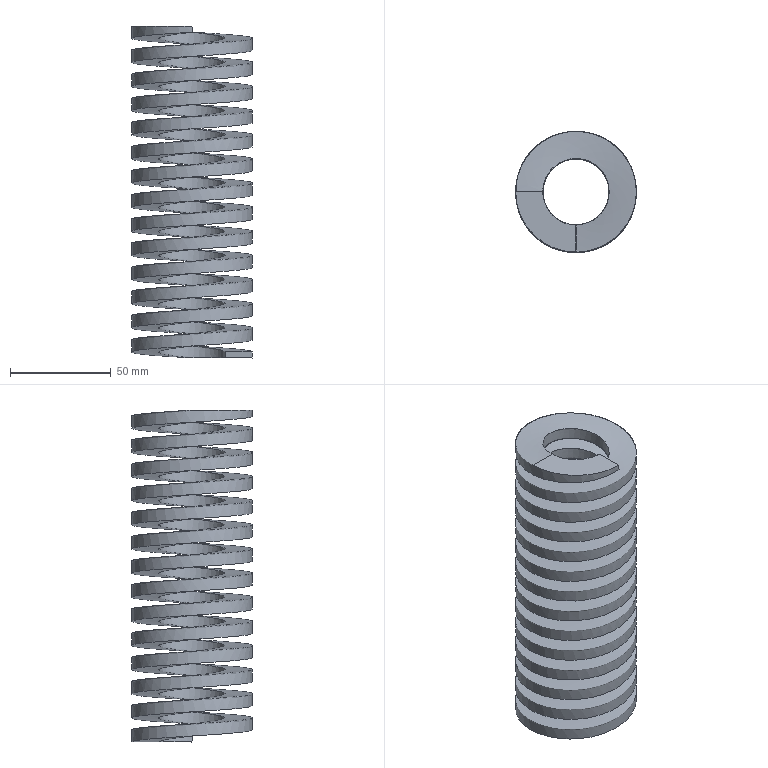Part | STEP file | E016017503 | 1 solid | 6 faces | volume 163409 mm3 | plane 4 | spline 2